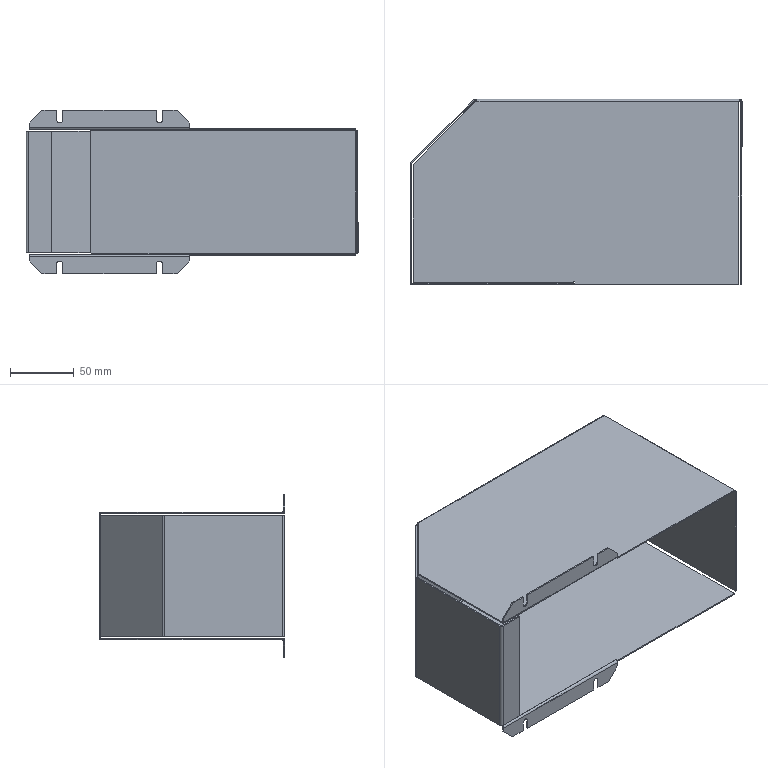Part | SolidWorks | features Chamfer 2, EdgeFlange 2, Extrusion 1, FlatPattern 1, HoleWzd 1, SheetMetal 1, SolidToSheetMetal 1 | 1 solid | 110 faces | box 260 x 145 x 128 mm | volume 125858 mm3 | plane 77 | cylinder 24 | spline 9 | commonest cylinder face diameters 1.473 x10 3.473 x8 4.8 x6